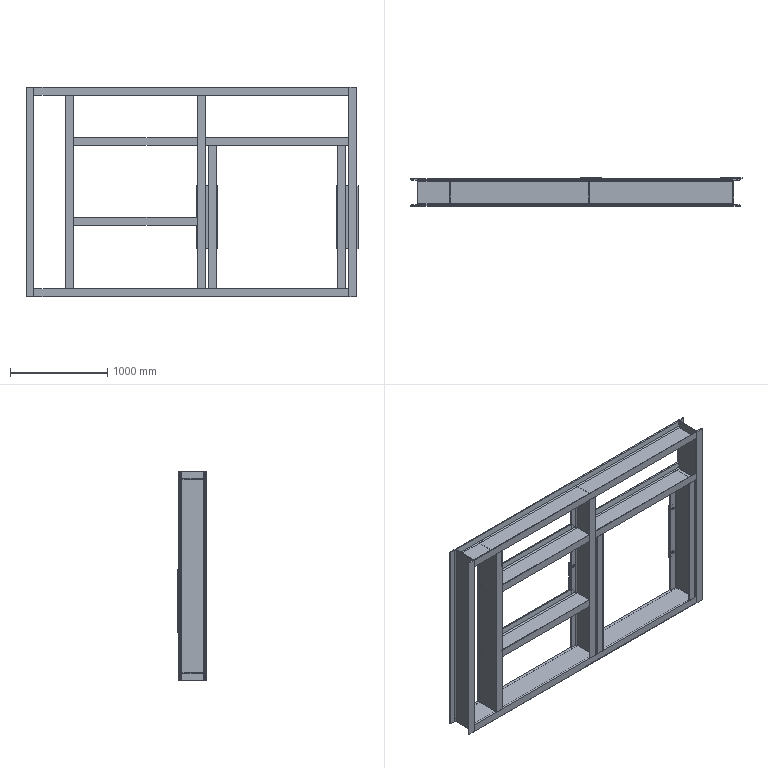Part | SolidWorks | features ICE 2, WeldMemberFeat 1, WeldmentFeature 1 | 13 solids | 222 faces | box 3413 x 292 x 2156 mm | volume 90885444 mm3 | plane 146 | cylinder 76 | commonest cylinder face diameters 32 x32 12.4 x22 25 x22